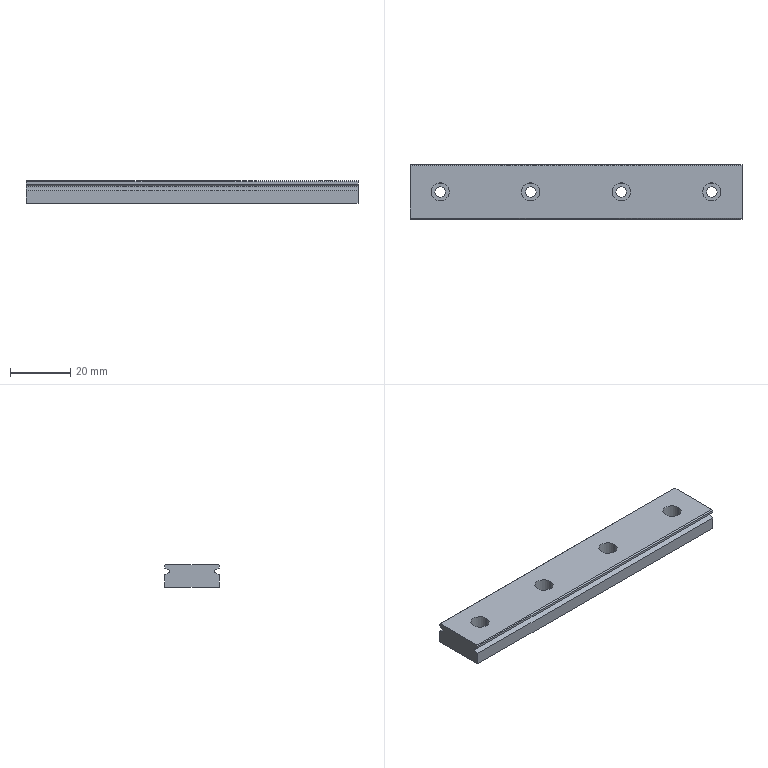Part | SolidWorks | features BaseBody 1, Cut 1 | 1 solid | 36 faces | box 110 x 18 x 7.5 mm | volume 13740 mm3 | plane 20 | cylinder 16 | commonest cylinder face diameters 3.5 x8 6 x8
STEP:
#1=CARTESIAN_POINT('',(-91.75,0.,0.));
#2=VERTEX_POINT('',#1);
#3=CARTESIAN_POINT('',(-88.25,0.,0.));
#4=VERTEX_POINT('',#3);
#5=CARTESIAN_POINT('',(-90.,0.,0.));
#6=DIRECTION('',(0.,0.,1.));
#7=DIRECTION('',(1.,0.,0.));
#8=AXIS2_PLACEMENT_3D('',#5,#6,#7);
#9=CIRCLE('',#8,1.75);
#10=EDGE_CURVE('',#2,#4,#9,.T.);
#11=ORIENTED_EDGE('',*,*,#10,.F.);
#12=CARTESIAN_POINT('',(-91.75,0.,3.));
#13=VERTEX_POINT('',#12);
#14=CARTESIAN_POINT('',(-91.75,0.,-1.163));
#15=DIRECTION('',(0.,0.,1.));
#16=VECTOR('',#15,1000.);
#17=LINE('',#14,#16);
#18=EDGE_CURVE('',#2,#13,#17,.T.);
#19=ORIENTED_EDGE('',*,*,#18,.T.);
#20=CARTESIAN_POINT('',(-88.25,0.,3.));
#21=VERTEX_POINT('',#20);
#22=CARTESIAN_POINT('',(-90.,0.,3.));
#23=DIRECTION('',(0.,0.,-1.));
#24=DIRECTION('',(1.,0.,0.));
#25=AXIS2_PLACEMENT_3D('',#22,#23,#24);
#26=CIRCLE('',#25,1.75);
#27=EDGE_CURVE('',#21,#13,#26,.T.);
#28=ORIENTED_EDGE('',*,*,#27,.F.);
#29=CARTESIAN_POINT('',(-88.25,0.,-1.163));
#30=DIRECTION('',(0.,0.,1.));
#31=VECTOR('',#30,1000.);
#32=LINE('',#29,#31);
#33=EDGE_CURVE('',#4,#21,#32,.T.);
#34=ORIENTED_EDGE('',*,*,#33,.F.);
#35=EDGE_LOOP('',(#11,#19,#28,#34));
#36=FACE_OUTER_BOUND('',#35,.T.);
#37=CARTESIAN_POINT('',(-90.,0.,-1.163));
#38=DIRECTION('',(0.,0.,1.));
#39=DIRECTION('',(1.,0.,0.));
#40=AXIS2_PLACEMENT_3D('',#37,#38,#39);
#41=CYLINDRICAL_SURFACE('',#40,1.75);
#42=ADVANCED_FACE('',(#36),#41,.F.);
#43=CARTESIAN_POINT('',(-61.75,0.,0.));
#44=VERTEX_POINT('',#43);
#45=CARTESIAN_POINT('',(-58.25,0.,0.));
#46=VERTEX_POINT('',#45);
#47=CARTESIAN_POINT('',(-60.,0.,0.));
#48=DIRECTION('',(0.,0.,1.));
#49=DIRECTION('',(1.,0.,0.));
#50=AXIS2_PLACEMENT_3D('',#47,#48,#49);
#51=CIRCLE('',#50,1.75);
#52=EDGE_CURVE('',#44,#46,#51,.T.);
#53=ORIENTED_EDGE('',*,*,#52,.F.);
#54=CARTESIAN_POINT('',(-61.75,0.,3.));
#55=VERTEX_POINT('',#54);
#56=CARTESIAN_POINT('',(-61.75,0.,-1.163));
#57=DIRECTION('',(0.,0.,1.));
#58=VECTOR('',#57,1000.);
#59=LINE('',#56,#58);
#60=EDGE_CURVE('',#44,#55,#59,.T.);
#61=ORIENTED_EDGE('',*,*,#60,.T.);
#62=CARTESIAN_POINT('',(-58.25,0.,3.));
#63=VERTEX_POINT('',#62);
#64=CARTESIAN_POINT('',(-60.,0.,3.));
#65=DIRECTION('',(0.,0.,-1.));
#66=DIRECTION('',(1.,0.,0.));
#67=AXIS2_PLACEMENT_3D('',#64,#65,#66);
#68=CIRCLE('',#67,1.75);
#69=EDGE_CURVE('',#63,#55,#68,.T.);
#70=ORIENTED_EDGE('',*,*,#69,.F.);
#71=CARTESIAN_POINT('',(-58.25,0.,-1.163));
#72=DIRECTION('',(0.,0.,1.));
#73=VECTOR('',#72,1000.);
#74=LINE('',#71,#73);
#75=EDGE_CURVE('',#46,#63,#74,.T.);
#76=ORIENTED_EDGE('',*,*,#75,.F.);
#77=EDGE_LOOP('',(#53,#61,#70,#76));
#78=FACE_OUTER_BOUND('',#77,.T.);
#79=CARTESIAN_POINT('',(-60.,0.,-1.163));
#80=DIRECTION('',(0.,0.,1.));
#81=DIRECTION('',(1.,0.,0.));
#82=AXIS2_PLACEMENT_3D('',#79,#80,#81);
#83=CYLINDRICAL_SURFACE('',#82,1.75);
#84=ADVANCED_FACE('',(#78),#83,.F.);
#85=CARTESIAN_POINT('',(-31.75,0.,0.));
#86=VERTEX_POINT('',#85);
#87=CARTESIAN_POINT('',(-28.25,0.,0.));
#88=VERTEX_POINT('',#87);
#89=CARTESIAN_POINT('',(-30.,0.,0.));
#90=DIRECTION('',(0.,0.,1.));
#91=DIRECTION('',(1.,0.,0.));
#92=AXIS2_PLACEMENT_3D('',#89,#90,#91);
#93=CIRCLE('',#92,1.75);
#94=EDGE_CURVE('',#86,#88,#93,.T.);
#95=ORIENTED_EDGE('',*,*,#94,.F.);
#96=CARTESIAN_POINT('',(-31.75,0.,3.));
#97=VERTEX_POINT('',#96);
#98=CARTESIAN_POINT('',(-31.75,0.,-1.163));
#99=DIRECTION('',(0.,0.,1.));
#100=VECTOR('',#99,1000.);
#101=LINE('',#98,#100);
#102=EDGE_CURVE('',#86,#97,#101,.T.);
#103=ORIENTED_EDGE('',*,*,#102,.T.);
#104=CARTESIAN_POINT('',(-28.25,0.,3.));
#105=VERTEX_POINT('',#104);
#106=CARTESIAN_POINT('',(-30.,0.,3.));
#107=DIRECTION('',(0.,0.,-1.));
#108=DIRECTION('',(1.,0.,0.));
#109=AXIS2_PLACEMENT_3D('',#106,#107,#108);
#110=CIRCLE('',#109,1.75);
#111=EDGE_CURVE('',#105,#97,#110,.T.);
#112=ORIENTED_EDGE('',*,*,#111,.F.);
#113=CARTESIAN_POINT('',(-28.25,0.,-1.163));
#114=DIRECTION('',(0.,0.,1.));
#115=VECTOR('',#114,1000.);
#116=LINE('',#113,#115);
#117=EDGE_CURVE('',#88,#105,#116,.T.);
#118=ORIENTED_EDGE('',*,*,#117,.F.);
#119=EDGE_LOOP('',(#95,#103,#112,#118));
#120=FACE_OUTER_BOUND('',#119,.T.);
#121=CARTESIAN_POINT('',(-30.,0.,-1.163));
#122=DIRECTION('',(0.,0.,1.));
#123=DIRECTION('',(1.,0.,0.));
#124=AXIS2_PLACEMENT_3D('',#121,#122,#123);
#125=CYLINDRICAL_SURFACE('',#124,1.75);
#126=ADVANCED_FACE('',(#120),#125,.F.);
#127=CARTESIAN_POINT('',(-1.75,0.,0.));
#128=VERTEX_POINT('',#127);
#129=CARTESIAN_POINT('',(1.75,0.,0.));
#130=VERTEX_POINT('',#129);
#131=CARTESIAN_POINT('',(0.,0.,0.));
#132=DIRECTION('',(0.,0.,1.));
#133=DIRECTION('',(1.,0.,0.));
#134=AXIS2_PLACEMENT_3D('',#131,#132,#133);
#135=CIRCLE('',#134,1.75);
#136=EDGE_CURVE('',#128,#130,#135,.T.);
#137=ORIENTED_EDGE('',*,*,#136,.F.);
#138=CARTESIAN_POINT('',(-1.75,0.,3.));
#139=VERTEX_POINT('',#138);
#140=CARTESIAN_POINT('',(-1.75,0.,1.5));
#141=DIRECTION('',(0.,0.,1.));
#142=VECTOR('',#141,1000.);
#143=LINE('',#140,#142);
#144=EDGE_CURVE('',#128,#139,#143,.T.);
#145=ORIENTED_EDGE('',*,*,#144,.T.);
#146=CARTESIAN_POINT('',(1.75,0.,3.));
#147=VERTEX_POINT('',#146);
#148=CARTESIAN_POINT('',(0.,0.,3.));
#149=DIRECTION('',(0.,0.,-1.));
#150=DIRECTION('',(1.,0.,0.));
#151=AXIS2_PLACEMENT_3D('',#148,#149,#150);
#152=CIRCLE('',#151,1.75);
#153=EDGE_CURVE('',#147,#139,#152,.T.);
#154=ORIENTED_EDGE('',*,*,#153,.F.);
#155=CARTESIAN_POINT('',(1.75,0.,1.5));
#156=DIRECTION('',(0.,0.,1.));
#157=VECTOR('',#156,1000.);
#158=LINE('',#155,#157);
#159=EDGE_CURVE('',#130,#147,#158,.T.);
#160=ORIENTED_EDGE('',*,*,#159,.F.);
#161=EDGE_LOOP('',(#137,#145,#154,#160));
#162=FACE_OUTER_BOUND('',#161,.T.);
#163=CARTESIAN_POINT('',(0.,0.,1.5));
#164=DIRECTION('',(0.,0.,1.));
#165=DIRECTION('',(1.,0.,0.));
#166=AXIS2_PLACEMENT_3D('',#163,#164,#165);
#167=CYLINDRICAL_SURFACE('',#166,1.75);
#168=ADVANCED_FACE('',(#162),#167,.F.);
#169=CARTESIAN_POINT('',(-93.,0.,3.));
#170=VERTEX_POINT('',#169);
#171=CARTESIAN_POINT('',(-87.,0.,3.));
#172=VERTEX_POINT('',#171);
#173=CARTESIAN_POINT('',(-90.,0.,3.));
#174=DIRECTION('',(0.,0.,1.));
#175=DIRECTION('',(1.,0.,0.));
#176=AXIS2_PLACEMENT_3D('',#173,#174,#175);
#177=CIRCLE('',#176,3.);
#178=EDGE_CURVE('',#170,#172,#177,.T.);
#179=ORIENTED_EDGE('',*,*,#178,.F.);
#180=CARTESIAN_POINT('',(-93.,0.,7.5));
#181=VERTEX_POINT('',#180);
#182=CARTESIAN_POINT('',(-93.,0.,-1.163));
#183=DIRECTION('',(0.,0.,1.));
#184=VECTOR('',#183,1000.);
#185=LINE('',#182,#184);
#186=EDGE_CURVE('',#170,#181,#185,.T.);
#187=ORIENTED_EDGE('',*,*,#186,.T.);
#188=CARTESIAN_POINT('',(-87.,0.,7.5));
#189=VERTEX_POINT('',#188);
#190=CARTESIAN_POINT('',(-90.,0.,7.5));
#191=DIRECTION('',(0.,0.,-1.));
#192=DIRECTION('',(1.,0.,0.));
#193=AXIS2_PLACEMENT_3D('',#190,#191,#192);
#194=CIRCLE('',#193,3.);
#195=EDGE_CURVE('',#189,#181,#194,.T.);
#196=ORIENTED_EDGE('',*,*,#195,.F.);
#197=CARTESIAN_POINT('',(-87.,0.,-1.163));
#198=DIRECTION('',(0.,0.,1.));
#199=VECTOR('',#198,1000.);
#200=LINE('',#197,#199);
#201=EDGE_CURVE('',#172,#189,#200,.T.);
#202=ORIENTED_EDGE('',*,*,#201,.F.);
#203=EDGE_LOOP('',(#179,#187,#196,#202));
#204=FACE_OUTER_BOUND('',#203,.T.);
#205=CARTESIAN_POINT('',(-90.,0.,-1.163));
#206=DIRECTION('',(0.,0.,1.));
#207=DIRECTION('',(1.,0.,0.));
#208=AXIS2_PLACEMENT_3D('',#205,#206,#207);
#209=CYLINDRICAL_SURFACE('',#208,3.);
#210=ADVANCED_FACE('',(#204),#209,.F.);
#211=CARTESIAN_POINT('',(-63.,0.,3.));
#212=VERTEX_POINT('',#211);
#213=CARTESIAN_POINT('',(-57.,0.,3.));
#214=VERTEX_POINT('',#213);
#215=CARTESIAN_POINT('',(-60.,0.,3.));
#216=DIRECTION('',(0.,0.,1.));
#217=DIRECTION('',(1.,0.,0.));
#218=AXIS2_PLACEMENT_3D('',#215,#216,#217);
#219=CIRCLE('',#218,3.);
#220=EDGE_CURVE('',#212,#214,#219,.T.);
#221=ORIENTED_EDGE('',*,*,#220,.F.);
#222=CARTESIAN_POINT('',(-63.,0.,7.5));
#223=VERTEX_POINT('',#222);
#224=CARTESIAN_POINT('',(-63.,0.,-1.163));
#225=DIRECTION('',(0.,0.,1.));
#226=VECTOR('',#225,1000.);
#227=LINE('',#224,#226);
#228=EDGE_CURVE('',#212,#223,#227,.T.);
#229=ORIENTED_EDGE('',*,*,#228,.T.);
#230=CARTESIAN_POINT('',(-57.,0.,7.5));
#231=VERTEX_POINT('',#230);
#232=CARTESIAN_POINT('',(-60.,0.,7.5));
#233=DIRECTION('',(0.,0.,-1.));
#234=DIRECTION('',(1.,0.,0.));
#235=AXIS2_PLACEMENT_3D('',#232,#233,#234);
#236=CIRCLE('',#235,3.);
#237=EDGE_CURVE('',#231,#223,#236,.T.);
#238=ORIENTED_EDGE('',*,*,#237,.F.);
#239=CARTESIAN_POINT('',(-57.,0.,-1.163));
#240=DIRECTION('',(0.,0.,1.));
#241=VECTOR('',#240,1000.);
#242=LINE('',#239,#241);
#243=EDGE_CURVE('',#214,#231,#242,.T.);
#244=ORIENTED_EDGE('',*,*,#243,.F.);
#245=EDGE_LOOP('',(#221,#229,#238,#244));
#246=FACE_OUTER_BOUND('',#245,.T.);
#247=CARTESIAN_POINT('',(-60.,0.,-1.163));
#248=DIRECTION('',(0.,0.,1.));
#249=DIRECTION('',(1.,0.,0.));
#250=AXIS2_PLACEMENT_3D('',#247,#248,#249);
#251=CYLINDRICAL_SURFACE('',#250,3.);
#252=ADVANCED_FACE('',(#246),#251,.F.);
#253=CARTESIAN_POINT('',(-33.,0.,3.));
#254=VERTEX_POINT('',#253);
#255=CARTESIAN_POINT('',(-27.,0.,3.));
#256=VERTEX_POINT('',#255);
#257=CARTESIAN_POINT('',(-30.,0.,3.));
#258=DIRECTION('',(0.,0.,1.));
#259=DIRECTION('',(1.,0.,0.));
#260=AXIS2_PLACEMENT_3D('',#257,#258,#259);
#261=CIRCLE('',#260,3.);
#262=EDGE_CURVE('',#254,#256,#261,.T.);
#263=ORIENTED_EDGE('',*,*,#262,.F.);
#264=CARTESIAN_POINT('',(-33.,0.,7.5));
#265=VERTEX_POINT('',#264);
#266=CARTESIAN_POINT('',(-33.,0.,-1.163));
#267=DIRECTION('',(0.,0.,1.));
#268=VECTOR('',#267,1000.);
#269=LINE('',#266,#268);
#270=EDGE_CURVE('',#254,#265,#269,.T.);
#271=ORIENTED_EDGE('',*,*,#270,.T.);
#272=CARTESIAN_POINT('',(-27.,0.,7.5));
#273=VERTEX_POINT('',#272);
#274=CARTESIAN_POINT('',(-30.,0.,7.5));
#275=DIRECTION('',(0.,0.,-1.));
#276=DIRECTION('',(1.,0.,0.));
#277=AXIS2_PLACEMENT_3D('',#274,#275,#276);
#278=CIRCLE('',#277,3.);
#279=EDGE_CURVE('',#273,#265,#278,.T.);
#280=ORIENTED_EDGE('',*,*,#279,.F.);
#281=CARTESIAN_POINT('',(-27.,0.,-1.163));
#282=DIRECTION('',(0.,0.,1.));
#283=VECTOR('',#282,1000.);
#284=LINE('',#281,#283);
#285=EDGE_CURVE('',#256,#273,#284,.T.);
#286=ORIENTED_EDGE('',*,*,#285,.F.);
#287=EDGE_LOOP('',(#263,#271,#280,#286));
#288=FACE_OUTER_BOUND('',#287,.T.);
#289=CARTESIAN_POINT('',(-30.,0.,-1.163));
#290=DIRECTION('',(0.,0.,1.));
#291=DIRECTION('',(1.,0.,0.));
#292=AXIS2_PLACEMENT_3D('',#289,#290,#291);
#293=CYLINDRICAL_SURFACE('',#292,3.);
#294=ADVANCED_FACE('',(#288),#293,.F.);
#295=CARTESIAN_POINT('',(3.,0.,7.5));
#296=VERTEX_POINT('',#295);
#297=CARTESIAN_POINT('',(-3.,0.,7.5));
#298=VERTEX_POINT('',#297);
#299=CARTESIAN_POINT('',(0.,0.,7.5));
#300=DIRECTION('',(0.,0.,-1.));
#301=DIRECTION('',(-1.,0.,0.));
#302=AXIS2_PLACEMENT_3D('',#299,#300,#301);
#303=CIRCLE('',#302,3.);
#304=EDGE_CURVE('',#296,#298,#303,.T.);
#305=ORIENTED_EDGE('',*,*,#304,.F.);
#306=CARTESIAN_POINT('',(3.,0.,3.));
#307=VERTEX_POINT('',#306);
#308=CARTESIAN_POINT('',(3.,0.,5.25));
#309=DIRECTION('',(0.,0.,-1.));
#310=VECTOR('',#309,1000.);
#311=LINE('',#308,#310);
#312=EDGE_CURVE('',#296,#307,#311,.T.);
#313=ORIENTED_EDGE('',*,*,#312,.T.);
#314=CARTESIAN_POINT('',(-3.,0.,3.));
#315=VERTEX_POINT('',#314);
#316=CARTESIAN_POINT('',(0.,0.,3.));
#317=DIRECTION('',(0.,0.,-1.));
#318=DIRECTION('',(-1.,0.,0.));
#319=AXIS2_PLACEMENT_3D('',#316,#317,#318);
#320=CIRCLE('',#319,3.);
#321=EDGE_CURVE('',#307,#315,#320,.T.);
#322=ORIENTED_EDGE('',*,*,#321,.T.);
#323=CARTESIAN_POINT('',(-3.,0.,5.25));
#324=DIRECTION('',(0.,0.,-1.));
#325=VECTOR('',#324,1000.);
#326=LINE('',#323,#325);
#327=EDGE_CURVE('',#298,#315,#326,.T.);
#328=ORIENTED_EDGE('',*,*,#327,.F.);
#329=EDGE_LOOP('',(#305,#313,#322,#328));
#330=FACE_OUTER_BOUND('',#329,.T.);
#331=CARTESIAN_POINT('',(0.,0.,5.25));
#332=DIRECTION('',(0.,0.,-1.));
#333=DIRECTION('',(-1.,0.,0.));
#334=AXIS2_PLACEMENT_3D('',#331,#332,#333);
#335=CYLINDRICAL_SURFACE('',#334,3.);
#336=ADVANCED_FACE('',(#330),#335,.F.);
#337=CARTESIAN_POINT('',(10.,-9.,0.));
#338=VERTEX_POINT('',#337);
#339=CARTESIAN_POINT('',(10.,9.,0.));
#340=VERTEX_POINT('',#339);
#341=CARTESIAN_POINT('',(10.,0.,0.));
#342=DIRECTION('',(0.,1.,0.));
#343=VECTOR('',#342,1000.);
#344=LINE('',#341,#343);
#345=EDGE_CURVE('',#338,#340,#344,.T.);
#346=ORIENTED_EDGE('',*,*,#345,.F.);
#347=CARTESIAN_POINT('',(-100.,-9.,0.));
#348=VERTEX_POINT('',#347);
#349=CARTESIAN_POINT('',(-10.,-9.,0.));
#350=DIRECTION('',(-1.,0.,0.));
#351=VECTOR('',#350,1000.);
#352=LINE('',#349,#351);
#353=EDGE_CURVE('',#338,#348,#352,.T.);
#354=ORIENTED_EDGE('',*,*,#353,.T.);
#355=CARTESIAN_POINT('',(-100.,9.,0.));
#356=VERTEX_POINT('',#355);
#357=CARTESIAN_POINT('',(-100.,0.,0.));
#358=DIRECTION('',(0.,1.,0.));
#359=VECTOR('',#358,1000.);
#360=LINE('',#357,#359);
#361=EDGE_CURVE('',#348,#356,#360,.T.);
#362=ORIENTED_EDGE('',*,*,#361,.T.);
#363=CARTESIAN_POINT('',(-10.,9.,0.));
#364=DIRECTION('',(1.,0.,0.));
#365=VECTOR('',#364,1000.);
#366=LINE('',#363,#365);
#367=EDGE_CURVE('',#356,#340,#366,.T.);
#368=ORIENTED_EDGE('',*,*,#367,.T.);
#369=EDGE_LOOP('',(#346,#354,#362,#368));
#370=FACE_OUTER_BOUND('',#369,.T.);
#371=CARTESIAN_POINT('',(-90.,0.,0.));
#372=DIRECTION('',(0.,0.,1.));
#373=DIRECTION('',(1.,0.,0.));
#374=AXIS2_PLACEMENT_3D('',#371,#372,#373);
#375=CIRCLE('',#374,1.75);
#376=EDGE_CURVE('',#4,#2,#375,.T.);
#377=ORIENTED_EDGE('',*,*,#376,.T.);
#378=ORIENTED_EDGE('',*,*,#10,.T.);
#379=EDGE_LOOP('',(#377,#378));
#380=FACE_BOUND('',#379,.T.);
#381=CARTESIAN_POINT('',(-60.,0.,0.));
#382=DIRECTION('',(0.,0.,1.));
#383=DIRECTION('',(1.,0.,0.));
#384=AXIS2_PLACEMENT_3D('',#381,#382,#383);
#385=CIRCLE('',#384,1.75);
#386=EDGE_CURVE('',#46,#44,#385,.T.);
#387=ORIENTED_EDGE('',*,*,#386,.T.);
#388=ORIENTED_EDGE('',*,*,#52,.T.);
#389=EDGE_LOOP('',(#387,#388));
#390=FACE_BOUND('',#389,.T.);
#391=CARTESIAN_POINT('',(-30.,0.,0.));
#392=DIRECTION('',(0.,0.,1.));
#393=DIRECTION('',(1.,0.,0.));
#394=AXIS2_PLACEMENT_3D('',#391,#392,#393);
#395=CIRCLE('',#394,1.75);
#396=EDGE_CURVE('',#88,#86,#395,.T.);
#397=ORIENTED_EDGE('',*,*,#396,.T.);
#398=ORIENTED_EDGE('',*,*,#94,.T.);
#399=EDGE_LOOP('',(#397,#398));
#400=FACE_BOUND('',#399,.T.);
#401=CARTESIAN_POINT('',(0.,0.,0.));
#402=DIRECTION('',(0.,0.,1.));
#403=DIRECTION('',(1.,0.,0.));
#404=AXIS2_PLACEMENT_3D('',#401,#402,#403);
#405=CIRCLE('',#404,1.75);
#406=EDGE_CURVE('',#130,#128,#405,.T.);
#407=ORIENTED_EDGE('',*,*,#406,.T.);
#408=ORIENTED_EDGE('',*,*,#136,.T.);
#409=EDGE_LOOP('',(#407,#408));
#410=FACE_BOUND('',#409,.T.);
#411=CARTESIAN_POINT('',(-10.,0.,0.));
#412=DIRECTION('',(0.,0.,-1.));
#413=DIRECTION('',(-1.,0.,0.));
#414=AXIS2_PLACEMENT_3D('',#411,#412,#413);
#415=PLANE('',#414);
#416=ADVANCED_FACE('',(#370,#380,#390,#400,#410),#415,.T.);
#417=ORIENTED_EDGE('',*,*,#18,.F.);
#418=ORIENTED_EDGE('',*,*,#376,.F.);
#419=ORIENTED_EDGE('',*,*,#33,.T.);
#420=CARTESIAN_POINT('',(-90.,0.,3.));
#421=DIRECTION('',(0.,0.,-1.));
#422=DIRECTION('',(1.,0.,0.));
#423=AXIS2_PLACEMENT_3D('',#420,#421,#422);
#424=CIRCLE('',#423,1.75);
#425=EDGE_CURVE('',#13,#21,#424,.T.);
#426=ORIENTED_EDGE('',*,*,#425,.F.);
#427=EDGE_LOOP('',(#417,#418,#419,#426));
#428=FACE_OUTER_BOUND('',#427,.T.);
#429=CARTESIAN_POINT('',(-90.,0.,-1.163));
#430=DIRECTION('',(0.,0.,1.));
#431=DIRECTION('',(1.,0.,0.));
#432=AXIS2_PLACEMENT_3D('',#429,#430,#431);
#433=CYLINDRICAL_SURFACE('',#432,1.75);
#434=ADVANCED_FACE('',(#428),#433,.F.);
#435=ORIENTED_EDGE('',*,*,#60,.F.);
#436=ORIENTED_EDGE('',*,*,#386,.F.);
#437=ORIENTED_EDGE('',*,*,#75,.T.);
#438=CARTESIAN_POINT('',(-60.,0.,3.));
#439=DIRECTION('',(0.,0.,-1.));
#440=DIRECTION('',(1.,0.,0.));
#441=AXIS2_PLACEMENT_3D('',#438,#439,#440);
#442=CIRCLE('',#441,1.75);
#443=EDGE_CURVE('',#55,#63,#442,.T.);
#444=ORIENTED_EDGE('',*,*,#443,.F.);
#445=EDGE_LOOP('',(#435,#436,#437,#444));
#446=FACE_OUTER_BOUND('',#445,.T.);
#447=CARTESIAN_POINT('',(-60.,0.,-1.163));
#448=DIRECTION('',(0.,0.,1.));
#449=DIRECTION('',(1.,0.,0.));
#450=AXIS2_PLACEMENT_3D('',#447,#448,#449);
#451=CYLINDRICAL_SURFACE('',#450,1.75);
#452=ADVANCED_FACE('',(#446),#451,.F.);
#453=ORIENTED_EDGE('',*,*,#102,.F.);
#454=ORIENTED_EDGE('',*,*,#396,.F.);
#455=ORIENTED_EDGE('',*,*,#117,.T.);
#456=CARTESIAN_POINT('',(-30.,0.,3.));
#457=DIRECTION('',(0.,0.,-1.));
#458=DIRECTION('',(1.,0.,0.));
#459=AXIS2_PLACEMENT_3D('',#456,#457,#458);
#460=CIRCLE('',#459,1.75);
#461=EDGE_CURVE('',#97,#105,#460,.T.);
#462=ORIENTED_EDGE('',*,*,#461,.F.);
#463=EDGE_LOOP('',(#453,#454,#455,#462));
#464=FACE_OUTER_BOUND('',#463,.T.);
#465=CARTESIAN_POINT('',(-30.,0.,-1.163));
#466=DIRECTION('',(0.,0.,1.));
#467=DIRECTION('',(1.,0.,0.));
#468=AXIS2_PLACEMENT_3D('',#465,#466,#467);
#469=CYLINDRICAL_SURFACE('',#468,1.75);
#470=ADVANCED_FACE('',(#464),#469,.F.);
#471=ORIENTED_EDGE('',*,*,#144,.F.);
#472=ORIENTED_EDGE('',*,*,#406,.F.);
#473=ORIENTED_EDGE('',*,*,#159,.T.);
#474=CARTESIAN_POINT('',(0.,0.,3.));
#475=DIRECTION('',(0.,0.,-1.));
#476=DIRECTION('',(1.,0.,0.));
#477=AXIS2_PLACEMENT_3D('',#474,#475,#476);
#478=CIRCLE('',#477,1.75);
#479=EDGE_CURVE('',#139,#147,#478,.T.);
#480=ORIENTED_EDGE('',*,*,#479,.F.);
#481=EDGE_LOOP('',(#471,#472,#473,#480));
#482=FACE_OUTER_BOUND('',#481,.T.);
#483=CARTESIAN_POINT('',(0.,0.,1.5));
#484=DIRECTION('',(0.,0.,1.));
#485=DIRECTION('',(1.,0.,0.));
#486=AXIS2_PLACEMENT_3D('',#483,#484,#485);
#487=CYLINDRICAL_SURFACE('',#486,1.75);
#488=ADVANCED_FACE('',(#482),#487,.F.);
#489=CARTESIAN_POINT('',(10.,9.,4.2));
#490=VERTEX_POINT('',#489);
#491=CARTESIAN_POINT('',(10.,9.,4.2));
#492=DIRECTION('',(0.,0.,1.));
#493=VECTOR('',#492,1000.);
#494=LINE('',#491,#493);
#495=EDGE_CURVE('',#340,#490,#494,.T.);
#496=ORIENTED_EDGE('',*,*,#495,.F.);
#497=ORIENTED_EDGE('',*,*,#367,.F.);
#498=CARTESIAN_POINT('',(-100.,9.,4.2));
#499=VERTEX_POINT('',#498);
#500=CARTESIAN_POINT('',(-100.,9.,4.2));
#501=DIRECTION('',(0.,0.,1.));
#502=VECTOR('',#501,1000.);
#503=LINE('',#500,#502);
#504=EDGE_CURVE('',#356,#499,#503,.T.);
#505=ORIENTED_EDGE('',*,*,#504,.T.);
#506=CARTESIAN_POINT('',(-10.,9.,4.2));
#507=DIRECTION('',(1.,0.,0.));
#508=VECTOR('',#507,1000.);
#509=LINE('',#506,#508);
#510=EDGE_CURVE('',#499,#490,#509,.T.);
#511=ORIENTED_EDGE('',*,*,#510,.T.);
#512=EDGE_LOOP('',(#496,#497,#505,#511));
#513=FACE_OUTER_BOUND('',#512,.T.);
#514=CARTESIAN_POINT('',(-10.,9.,4.2));
#515=DIRECTION('',(0.,1.,0.));
#516=DIRECTION('',(0.,0.,1.));
#517=AXIS2_PLACEMENT_3D('',#514,#515,#516);
#518=PLANE('',#517);
#519=ADVANCED_FACE('',(#513),#518,.T.);
#520=ORIENTED_EDGE('',*,*,#504,.F.);
#521=ORIENTED_EDGE('',*,*,#361,.F.);
#522=CARTESIAN_POINT('',(-100.,-9.,4.2));
#523=VERTEX_POINT('',#522);
#524=CARTESIAN_POINT('',(-100.,-9.,0.));
#525=DIRECTION('',(0.,0.,1.));
#526=VECTOR('',#525,1000.);
#527=LINE('',#524,#526);
#528=EDGE_CURVE('',#348,#523,#527,.T.);
#529=ORIENTED_EDGE('',*,*,#528,.T.);
#530=CARTESIAN_POINT('',(-100.,-7.5,4.95));
#531=VERTEX_POINT('',#530);
#532=CARTESIAN_POINT('',(-100.,-9.,4.2));
#533=DIRECTION('',(0.,-0.8944,-0.4472));
#534=VECTOR('',#533,1000.);
#535=LINE('',#532,#534);
#536=EDGE_CURVE('',#531,#523,#535,.T.);
#537=ORIENTED_EDGE('',*,*,#536,.F.);
#538=CARTESIAN_POINT('',(-100.,-7.5,5.625));
#539=VERTEX_POINT('',#538);
#540=CARTESIAN_POINT('',(-100.,-7.5,4.95));
#541=DIRECTION('',(0.,0.,-1.));
#542=VECTOR('',#541,1000.);
#543=LINE('',#540,#542);
#544=EDGE_CURVE('',#539,#531,#543,.T.);
#545=ORIENTED_EDGE('',*,*,#544,.F.);
#546=CARTESIAN_POINT('',(-100.,-9.,6.375));
#547=VERTEX_POINT('',#546);
#548=CARTESIAN_POINT('',(-100.,-7.5,5.625));
#549=DIRECTION('',(0.,0.8944,-0.4472));
#550=VECTOR('',#549,1000.);
#551=LINE('',#548,#550);
#552=EDGE_CURVE('',#547,#539,#551,.T.);
#553=ORIENTED_EDGE('',*,*,#552,.F.);
#554=CARTESIAN_POINT('',(-100.,-9.,7.125));
#555=VERTEX_POINT('',#554);
#556=CARTESIAN_POINT('',(-100.,-9.,6.375));
#557=DIRECTION('',(0.,0.,-1.));
#558=VECTOR('',#557,1000.);
#559=LINE('',#556,#558);
#560=EDGE_CURVE('',#555,#547,#559,.T.);
#561=ORIENTED_EDGE('',*,*,#560,.F.);
#562=CARTESIAN_POINT('',(-100.,-8.625,7.5));
#563=VERTEX_POINT('',#562);
#564=CARTESIAN_POINT('',(-100.,-9.,7.125));
#565=DIRECTION('',(0.,-0.7071,-0.7071));
#566=VECTOR('',#565,1000.);
#567=LINE('',#564,#566);
#568=EDGE_CURVE('',#563,#555,#567,.T.);
#569=ORIENTED_EDGE('',*,*,#568,.F.);
#570=CARTESIAN_POINT('',(-100.,8.625,7.5));
#571=VERTEX_POINT('',#570);
#572=CARTESIAN_POINT('',(-100.,0.,7.5));
#573=DIRECTION('',(0.,1.,0.));
#574=VECTOR('',#573,1000.);
#575=LINE('',#572,#574);
#576=EDGE_CURVE('',#563,#571,#575,.T.);
#577=ORIENTED_EDGE('',*,*,#576,.T.);
#578=CARTESIAN_POINT('',(-100.,9.,7.125));
#579=VERTEX_POINT('',#578);
#580=CARTESIAN_POINT('',(-100.,8.625,7.5));
#581=DIRECTION('',(0.,-0.7071,0.7071));
#582=VECTOR('',#581,1000.);
#583=LINE('',#580,#582);
#584=EDGE_CURVE('',#579,#571,#583,.T.);
#585=ORIENTED_EDGE('',*,*,#584,.F.);
#586=CARTESIAN_POINT('',(-100.,9.,6.375));
#587=VERTEX_POINT('',#586);
#588=CARTESIAN_POINT('',(-100.,9.,7.125));
#589=DIRECTION('',(0.,0.,1.));
#590=VECTOR('',#589,1000.);
#591=LINE('',#588,#590);
#592=EDGE_CURVE('',#587,#579,#591,.T.);
#593=ORIENTED_EDGE('',*,*,#592,.F.);
#594=CARTESIAN_POINT('',(-100.,7.5,5.625));
#595=VERTEX_POINT('',#594);
#596=CARTESIAN_POINT('',(-100.,9.,6.375));
#597=DIRECTION('',(0.,0.8944,0.4472));
#598=VECTOR('',#597,1000.);
#599=LINE('',#596,#598);
#600=EDGE_CURVE('',#595,#587,#599,.T.);
#601=ORIENTED_EDGE('',*,*,#600,.F.);
#602=CARTESIAN_POINT('',(-100.,7.5,4.95));
#603=VERTEX_POINT('',#602);
#604=CARTESIAN_POINT('',(-100.,7.5,5.625));
#605=DIRECTION('',(0.,0.,1.));
#606=VECTOR('',#605,1000.);
#607=LINE('',#604,#606);
#608=EDGE_CURVE('',#603,#595,#607,.T.);
#609=ORIENTED_EDGE('',*,*,#608,.F.);
#610=CARTESIAN_POINT('',(-100.,7.5,4.95));
#611=DIRECTION('',(0.,0.8944,-0.4472));
#612=VECTOR('',#611,1000.);
#613=LINE('',#610,#612);
#614=EDGE_CURVE('',#603,#499,#613,.T.);
#615=ORIENTED_EDGE('',*,*,#614,.T.);
#616=EDGE_LOOP('',(#520,#521,#529,#537,#545,#553,#561,#569,#577,#585,#593,#601,#609,#615));
#617=FACE_OUTER_BOUND('',#616,.T.);
#618=CARTESIAN_POINT('',(-100.,0.,0.));
#619=DIRECTION('',(-1.,0.,0.));
#620=DIRECTION('',(0.,0.,1.));
#621=AXIS2_PLACEMENT_3D('',#618,#619,#620);
#622=PLANE('',#621);
#623=ADVANCED_FACE('',(#617),#622,.T.);
#624=CARTESIAN_POINT('',(10.,-9.,4.2));
#625=VERTEX_POINT('',#624);
#626=CARTESIAN_POINT('',(10.,-9.,0.));
#627=DIRECTION('',(0.,0.,-1.));
#628=VECTOR('',#627,1000.);
#629=LINE('',#626,#628);
#630=EDGE_CURVE('',#625,#338,#629,.T.);
#631=ORIENTED_EDGE('',*,*,#630,.F.);
#632=CARTESIAN_POINT('',(-10.,-9.,4.2));
#633=DIRECTION('',(-1.,0.,0.));
#634=VECTOR('',#633,1000.);
#635=LINE('',#632,#634);
#636=EDGE_CURVE('',#625,#523,#635,.T.);
#637=ORIENTED_EDGE('',*,*,#636,.T.);
#638=ORIENTED_EDGE('',*,*,#528,.F.);
#639=ORIENTED_EDGE('',*,*,#353,.F.);
#640=EDGE_LOOP('',(#631,#637,#638,#639));
#641=FACE_OUTER_BOUND('',#640,.T.);
#642=CARTESIAN_POINT('',(-10.,-9.,0.));
#643=DIRECTION('',(0.,-1.,0.));
#644=DIRECTION('',(0.,0.,-1.));
#645=AXIS2_PLACEMENT_3D('',#642,#643,#644);
#646=PLANE('',#645);
#647=ADVANCED_FACE('',(#641),#646,.T.);
#648=ORIENTED_EDGE('',*,*,#27,.T.);
#649=ORIENTED_EDGE('',*,*,#425,.T.);
#650=EDGE_LOOP('',(#648,#649));
#651=FACE_BOUND('',#650,.T.);
#652=CARTESIAN_POINT('',(-90.,0.,3.));
#653=DIRECTION('',(0.,0.,1.));
#654=DIRECTION('',(1.,0.,0.));
#655=AXIS2_PLACEMENT_3D('',#652,#653,#654);
#656=CIRCLE('',#655,3.);
#657=EDGE_CURVE('',#172,#170,#656,.T.);
#658=ORIENTED_EDGE('',*,*,#657,.T.);
#659=ORIENTED_EDGE('',*,*,#178,.T.);
#660=EDGE_LOOP('',(#658,#659));
#661=FACE_OUTER_BOUND('',#660,.T.);
#662=CARTESIAN_POINT('',(-90.,0.,3.));
#663=DIRECTION('',(0.,0.,1.));
#664=DIRECTION('',(1.,0.,0.));
#665=AXIS2_PLACEMENT_3D('',#662,#663,#664);
#666=PLANE('',#665);
#667=ADVANCED_FACE('',(#651,#661),#666,.T.);
#668=ORIENTED_EDGE('',*,*,#69,.T.);
#669=ORIENTED_EDGE('',*,*,#443,.T.);
#670=EDGE_LOOP('',(#668,#669));
#671=FACE_BOUND('',#670,.T.);
#672=CARTESIAN_POINT('',(-60.,0.,3.));
#673=DIRECTION('',(0.,0.,1.));
#674=DIRECTION('',(1.,0.,0.));
#675=AXIS2_PLACEMENT_3D('',#672,#673,#674);
#676=CIRCLE('',#675,3.);
#677=EDGE_CURVE('',#214,#212,#676,.T.);
#678=ORIENTED_EDGE('',*,*,#677,.T.);
#679=ORIENTED_EDGE('',*,*,#220,.T.);
#680=EDGE_LOOP('',(#678,#679));
#681=FACE_OUTER_BOUND('',#680,.T.);
#682=CARTESIAN_POINT('',(-60.,0.,3.));
#683=DIRECTION('',(0.,0.,1.));
#684=DIRECTION('',(1.,0.,0.));
#685=AXIS2_PLACEMENT_3D('',#682,#683,#684);
#686=PLANE('',#685);
#687=ADVANCED_FACE('',(#671,#681),#686,.T.);
#688=ORIENTED_EDGE('',*,*,#111,.T.);
#689=ORIENTED_EDGE('',*,*,#461,.T.);
#690=EDGE_LOOP('',(#688,#689));
#691=FACE_BOUND('',#690,.T.);
#692=CARTESIAN_POINT('',(-30.,0.,3.));
#693=DIRECTION('',(0.,0.,1.));
#694=DIRECTION('',(1.,0.,0.));
#695=AXIS2_PLACEMENT_3D('',#692,#693,#694);
#696=CIRCLE('',#695,3.);
#697=EDGE_CURVE('',#256,#254,#696,.T.);
#698=ORIENTED_EDGE('',*,*,#697,.T.);
#699=ORIENTED_EDGE('',*,*,#262,.T.);
#700=EDGE_LOOP('',(#698,#699));
#701=FACE_OUTER_BOUND('',#700,.T.);
#702=CARTESIAN_POINT('',(-30.,0.,3.));
#703=DIRECTION('',(0.,0.,1.));
#704=DIRECTION('',(1.,0.,0.));
#705=AXIS2_PLACEMENT_3D('',#702,#703,#704);
#706=PLANE('',#705);
#707=ADVANCED_FACE('',(#691,#701),#706,.T.);
#708=ORIENTED_EDGE('',*,*,#153,.T.);
#709=ORIENTED_EDGE('',*,*,#479,.T.);
#710=EDGE_LOOP('',(#708,#709));
#711=FACE_BOUND('',#710,.T.);
#712=CARTESIAN_POINT('',(0.,0.,3.));
#713=DIRECTION('',(0.,0.,-1.));
#714=DIRECTION('',(-1.,0.,0.));
#715=AXIS2_PLACEMENT_3D('',#712,#713,#714);
#716=CIRCLE('',#715,3.);
#717=EDGE_CURVE('',#315,#307,#716,.T.);
#718=ORIENTED_EDGE('',*,*,#717,.F.);
#719=ORIENTED_EDGE('',*,*,#321,.F.);
#720=EDGE_LOOP('',(#718,#719));
#721=FACE_OUTER_BOUND('',#720,.T.);
#722=CARTESIAN_POINT('',(0.,0.,3.));
#723=DIRECTION('',(0.,0.,-1.));
#724=DIRECTION('',(-1.,0.,0.));
#725=AXIS2_PLACEMENT_3D('',#722,#723,#724);
#726=PLANE('',#725);
#727=ADVANCED_FACE('',(#711,#721),#726,.F.);
#728=CARTESIAN_POINT('',(10.,7.5,4.95));
#729=VERTEX_POINT('',#728);
#730=CARTESIAN_POINT('',(10.,7.5,4.95));
#731=DIRECTION('',(0.,-0.8944,0.4472));
#732=VECTOR('',#731,1000.);
#733=LINE('',#730,#732);
#734=EDGE_CURVE('',#490,#729,#733,.T.);
#735=ORIENTED_EDGE('',*,*,#734,.F.);
#736=ORIENTED_EDGE('',*,*,#510,.F.);
#737=ORIENTED_EDGE('',*,*,#614,.F.);
#738=CARTESIAN_POINT('',(-10.,7.5,4.95));
#739=DIRECTION('',(1.,0.,0.));
#740=VECTOR('',#739,1000.);
#741=LINE('',#738,#740);
#742=EDGE_CURVE('',#603,#729,#741,.T.);
#743=ORIENTED_EDGE('',*,*,#742,.T.);
#744=EDGE_LOOP('',(#735,#736,#737,#743));
#745=FACE_OUTER_BOUND('',#744,.T.);
#746=CARTESIAN_POINT('',(-10.,7.5,4.95));
#747=DIRECTION('',(0.,0.4472,0.8944));
#748=DIRECTION('',(0.,-0.8944,0.4472));
#749=AXIS2_PLACEMENT_3D('',#746,#747,#748);
#750=PLANE('',#749);
#751=ADVANCED_FACE('',(#745),#750,.T.);
#752=CARTESIAN_POINT('',(10.,8.625,7.5));
#753=VERTEX_POINT('',#752);
#754=CARTESIAN_POINT('',(10.,-8.625,7.5));
#755=VERTEX_POINT('',#754);
#756=CARTESIAN_POINT('',(10.,19.873,7.5));
#757=DIRECTION('',(0.,-1.,0.));
#758=VECTOR('',#757,1000.);
#759=LINE('',#756,#758);
#760=EDGE_CURVE('',#753,#755,#759,.T.);
#761=ORIENTED_EDGE('',*,*,#760,.F.);
#762=CARTESIAN_POINT('',(-10.,8.625,7.5));
#763=DIRECTION('',(-1.,0.,0.));
#764=VECTOR('',#763,1000.);
#765=LINE('',#762,#764);
#766=EDGE_CURVE('',#753,#571,#765,.T.);
#767=ORIENTED_EDGE('',*,*,#766,.T.);
#768=ORIENTED_EDGE('',*,*,#576,.F.);
#769=CARTESIAN_POINT('',(-10.,-8.625,7.5));
#770=DIRECTION('',(1.,0.,0.));
#771=VECTOR('',#770,1000.);
#772=LINE('',#769,#771);
#773=EDGE_CURVE('',#563,#755,#772,.T.);
#774=ORIENTED_EDGE('',*,*,#773,.T.);
#775=EDGE_LOOP('',(#761,#767,#768,#774));
#776=FACE_OUTER_BOUND('',#775,.T.);
#777=ORIENTED_EDGE('',*,*,#195,.T.);
#778=CARTESIAN_POINT('',(-90.,0.,7.5));
#779=DIRECTION('',(0.,0.,-1.));
#780=DIRECTION('',(1.,0.,0.));
#781=AXIS2_PLACEMENT_3D('',#778,#779,#780);
#782=CIRCLE('',#781,3.);
#783=EDGE_CURVE('',#181,#189,#782,.T.);
#784=ORIENTED_EDGE('',*,*,#783,.T.);
#785=EDGE_LOOP('',(#777,#784));
#786=FACE_BOUND('',#785,.T.);
#787=ORIENTED_EDGE('',*,*,#237,.T.);
#788=CARTESIAN_POINT('',(-60.,0.,7.5));
#789=DIRECTION('',(0.,0.,-1.));
#790=DIRECTION('',(1.,0.,0.));
#791=AXIS2_PLACEMENT_3D('',#788,#789,#790);
#792=CIRCLE('',#791,3.);
#793=EDGE_CURVE('',#223,#231,#792,.T.);
#794=ORIENTED_EDGE('',*,*,#793,.T.);
#795=EDGE_LOOP('',(#787,#794));
#796=FACE_BOUND('',#795,.T.);
#797=ORIENTED_EDGE('',*,*,#279,.T.);
#798=CARTESIAN_POINT('',(-30.,0.,7.5));
#799=DIRECTION('',(0.,0.,-1.));
#800=DIRECTION('',(1.,0.,0.));
#801=AXIS2_PLACEMENT_3D('',#798,#799,#800);
#802=CIRCLE('',#801,3.);
#803=EDGE_CURVE('',#265,#273,#802,.T.);
#804=ORIENTED_EDGE('',*,*,#803,.T.);
#805=EDGE_LOOP('',(#797,#804));
#806=FACE_BOUND('',#805,.T.);
#807=CARTESIAN_POINT('',(0.,0.,7.5));
#808=DIRECTION('',(0.,0.,-1.));
#809=DIRECTION('',(-1.,0.,0.));
#810=AXIS2_PLACEMENT_3D('',#807,#808,#809);
#811=CIRCLE('',#810,3.);
#812=EDGE_CURVE('',#298,#296,#811,.T.);
#813=ORIENTED_EDGE('',*,*,#812,.T.);
#814=ORIENTED_EDGE('',*,*,#304,.T.);
#815=EDGE_LOOP('',(#813,#814));
#816=FACE_BOUND('',#815,.T.);
#817=CARTESIAN_POINT('',(-10.,-8.625,7.5));
#818=DIRECTION('',(0.,0.,1.));
#819=DIRECTION('',(1.,0.,0.));
#820=AXIS2_PLACEMENT_3D('',#817,#818,#819);
#821=PLANE('',#820);
#822=ADVANCED_FACE('',(#776,#786,#796,#806,#816),#821,.T.);
#823=CARTESIAN_POINT('',(10.,-7.5,4.95));
#824=VERTEX_POINT('',#823);
#825=CARTESIAN_POINT('',(10.,-9.,4.2));
#826=DIRECTION('',(0.,-0.8944,-0.4472));
#827=VECTOR('',#826,1000.);
#828=LINE('',#825,#827);
#829=EDGE_CURVE('',#824,#625,#828,.T.);
#830=ORIENTED_EDGE('',*,*,#829,.F.);
#831=CARTESIAN_POINT('',(-10.,-7.5,4.95));
#832=DIRECTION('',(-1.,0.,0.));
#833=VECTOR('',#832,1000.);
#834=LINE('',#831,#833);
#835=EDGE_CURVE('',#824,#531,#834,.T.);
#836=ORIENTED_EDGE('',*,*,#835,.T.);
#837=ORIENTED_EDGE('',*,*,#536,.T.);
#838=ORIENTED_EDGE('',*,*,#636,.F.);
#839=EDGE_LOOP('',(#830,#836,#837,#838));
#840=FACE_OUTER_BOUND('',#839,.T.);
#841=CARTESIAN_POINT('',(-10.,-9.,4.2));
#842=DIRECTION('',(0.,-0.4472,0.8944));
#843=DIRECTION('',(0.,-0.8944,-0.4472));
#844=AXIS2_PLACEMENT_3D('',#841,#842,#843);
#845=PLANE('',#844);
#846=ADVANCED_FACE('',(#840),#845,.T.);
#847=ORIENTED_EDGE('',*,*,#186,.F.);
#848=ORIENTED_EDGE('',*,*,#657,.F.);
#849=ORIENTED_EDGE('',*,*,#201,.T.);
#850=ORIENTED_EDGE('',*,*,#783,.F.);
#851=EDGE_LOOP('',(#847,#848,#849,#850));
#852=FACE_OUTER_BOUND('',#851,.T.);
#853=CARTESIAN_POINT('',(-90.,0.,-1.163));
#854=DIRECTION('',(0.,0.,1.));
#855=DIRECTION('',(1.,0.,0.));
#856=AXIS2_PLACEMENT_3D('',#853,#854,#855);
#857=CYLINDRICAL_SURFACE('',#856,3.);
#858=ADVANCED_FACE('',(#852),#857,.F.);
#859=ORIENTED_EDGE('',*,*,#228,.F.);
#860=ORIENTED_EDGE('',*,*,#677,.F.);
#861=ORIENTED_EDGE('',*,*,#243,.T.);
#862=ORIENTED_EDGE('',*,*,#793,.F.);
#863=EDGE_LOOP('',(#859,#860,#861,#862));
#864=FACE_OUTER_BOUND('',#863,.T.);
#865=CARTESIAN_POINT('',(-60.,0.,-1.163));
#866=DIRECTION('',(0.,0.,1.));
#867=DIRECTION('',(1.,0.,0.));
#868=AXIS2_PLACEMENT_3D('',#865,#866,#867);
#869=CYLINDRICAL_SURFACE('',#868,3.);
#870=ADVANCED_FACE('',(#864),#869,.F.);
#871=ORIENTED_EDGE('',*,*,#270,.F.);
#872=ORIENTED_EDGE('',*,*,#697,.F.);
#873=ORIENTED_EDGE('',*,*,#285,.T.);
#874=ORIENTED_EDGE('',*,*,#803,.F.);
#875=EDGE_LOOP('',(#871,#872,#873,#874));
#876=FACE_OUTER_BOUND('',#875,.T.);
#877=CARTESIAN_POINT('',(-30.,0.,-1.163));
#878=DIRECTION('',(0.,0.,1.));
#879=DIRECTION('',(1.,0.,0.));
#880=AXIS2_PLACEMENT_3D('',#877,#878,#879);
#881=CYLINDRICAL_SURFACE('',#880,3.);
#882=ADVANCED_FACE('',(#876),#881,.F.);
#883=ORIENTED_EDGE('',*,*,#312,.F.);
#884=ORIENTED_EDGE('',*,*,#812,.F.);
#885=ORIENTED_EDGE('',*,*,#327,.T.);
#886=ORIENTED_EDGE('',*,*,#717,.T.);
#887=EDGE_LOOP('',(#883,#884,#885,#886));
#888=FACE_OUTER_BOUND('',#887,.T.);
#889=CARTESIAN_POINT('',(0.,0.,5.25));
#890=DIRECTION('',(0.,0.,-1.));
#891=DIRECTION('',(-1.,0.,0.));
#892=AXIS2_PLACEMENT_3D('',#889,#890,#891);
#893=CYLINDRICAL_SURFACE('',#892,3.);
#894=ADVANCED_FACE('',(#888),#893,.F.);
#895=CARTESIAN_POINT('',(10.,7.5,5.625));
#896=VERTEX_POINT('',#895);
#897=CARTESIAN_POINT('',(10.,7.5,5.625));
#898=DIRECTION('',(0.,0.,1.));
#899=VECTOR('',#898,1000.);
#900=LINE('',#897,#899);
#901=EDGE_CURVE('',#729,#896,#900,.T.);
#902=ORIENTED_EDGE('',*,*,#901,.F.);
#903=ORIENTED_EDGE('',*,*,#742,.F.);
#904=ORIENTED_EDGE('',*,*,#608,.T.);
#905=CARTESIAN_POINT('',(-10.,7.5,5.625));
#906=DIRECTION('',(1.,0.,0.));
#907=VECTOR('',#906,1000.);
#908=LINE('',#905,#907);
#909=EDGE_CURVE('',#595,#896,#908,.T.);
#910=ORIENTED_EDGE('',*,*,#909,.T.);
#911=EDGE_LOOP('',(#902,#903,#904,#910));
#912=FACE_OUTER_BOUND('',#911,.T.);
#913=CARTESIAN_POINT('',(-10.,7.5,5.625));
#914=DIRECTION('',(0.,1.,0.));
#915=DIRECTION('',(0.,0.,1.));
#916=AXIS2_PLACEMENT_3D('',#913,#914,#915);
#917=PLANE('',#916);
#918=ADVANCED_FACE('',(#912),#917,.T.);
#919=CARTESIAN_POINT('',(10.,-9.,7.125));
#920=VERTEX_POINT('',#919);
#921=CARTESIAN_POINT('',(10.,-9.,7.125));
#922=DIRECTION('',(0.,-0.7071,-0.7071));
#923=VECTOR('',#922,1000.);
#924=LINE('',#921,#923);
#925=EDGE_CURVE('',#755,#920,#924,.T.);
#926=ORIENTED_EDGE('',*,*,#925,.F.);
#927=ORIENTED_EDGE('',*,*,#773,.F.);
#928=ORIENTED_EDGE('',*,*,#568,.T.);
#929=CARTESIAN_POINT('',(-10.,-9.,7.125));
#930=DIRECTION('',(1.,0.,0.));
#931=VECTOR('',#930,1000.);
#932=LINE('',#929,#931);
#933=EDGE_CURVE('',#555,#920,#932,.T.);
#934=ORIENTED_EDGE('',*,*,#933,.T.);
#935=EDGE_LOOP('',(#926,#927,#928,#934));
#936=FACE_OUTER_BOUND('',#935,.T.);
#937=CARTESIAN_POINT('',(-10.,-9.,7.125));
#938=DIRECTION('',(0.,-0.7071,0.7071));
#939=DIRECTION('',(0.,-0.7071,-0.7071));
#940=AXIS2_PLACEMENT_3D('',#937,#938,#939);
#941=PLANE('',#940);
#942=ADVANCED_FACE('',(#936),#941,.T.);
#943=CARTESIAN_POINT('',(10.,9.,7.125));
#944=VERTEX_POINT('',#943);
#945=CARTESIAN_POINT('',(10.,8.625,7.5));
#946=DIRECTION('',(0.,-0.7071,0.7071));
#947=VECTOR('',#946,1000.);
#948=LINE('',#945,#947);
#949=EDGE_CURVE('',#944,#753,#948,.T.);
#950=ORIENTED_EDGE('',*,*,#949,.F.);
#951=CARTESIAN_POINT('',(-10.,9.,7.125));
#952=DIRECTION('',(-1.,0.,0.));
#953=VECTOR('',#952,1000.);
#954=LINE('',#951,#953);
#955=EDGE_CURVE('',#944,#579,#954,.T.);
#956=ORIENTED_EDGE('',*,*,#955,.T.);
#957=ORIENTED_EDGE('',*,*,#584,.T.);
#958=ORIENTED_EDGE('',*,*,#766,.F.);
#959=EDGE_LOOP('',(#950,#956,#957,#958));
#960=FACE_OUTER_BOUND('',#959,.T.);
#961=CARTESIAN_POINT('',(-10.,8.625,7.5));
#962=DIRECTION('',(0.,0.7071,0.7071));
#963=DIRECTION('',(0.,-0.7071,0.7071));
#964=AXIS2_PLACEMENT_3D('',#961,#962,#963);
#965=PLANE('',#964);
#966=ADVANCED_FACE('',(#960),#965,.T.);
#967=CARTESIAN_POINT('',(10.,-7.5,5.625));
#968=VERTEX_POINT('',#967);
#969=CARTESIAN_POINT('',(10.,-7.5,4.95));
#970=DIRECTION('',(0.,0.,-1.));
#971=VECTOR('',#970,1000.);
#972=LINE('',#969,#971);
#973=EDGE_CURVE('',#968,#824,#972,.T.);
#974=ORIENTED_EDGE('',*,*,#973,.F.);
#975=CARTESIAN_POINT('',(-10.,-7.5,5.625));
#976=DIRECTION('',(-1.,0.,0.));
#977=VECTOR('',#976,1000.);
#978=LINE('',#975,#977);
#979=EDGE_CURVE('',#968,#539,#978,.T.);
#980=ORIENTED_EDGE('',*,*,#979,.T.);
#981=ORIENTED_EDGE('',*,*,#544,.T.);
#982=ORIENTED_EDGE('',*,*,#835,.F.);
#983=EDGE_LOOP('',(#974,#980,#981,#982));
#984=FACE_OUTER_BOUND('',#983,.T.);
#985=CARTESIAN_POINT('',(-10.,-7.5,4.95));
#986=DIRECTION('',(0.,-1.,0.));
#987=DIRECTION('',(0.,0.,-1.));
#988=AXIS2_PLACEMENT_3D('',#985,#986,#987);
#989=PLANE('',#988);
#990=ADVANCED_FACE('',(#984),#989,.T.);
#991=CARTESIAN_POINT('',(10.,9.,6.375));
#992=VERTEX_POINT('',#991);
#993=CARTESIAN_POINT('',(10.,9.,6.375));
#994=DIRECTION('',(0.,0.8944,0.4472));
#995=VECTOR('',#994,1000.);
#996=LINE('',#993,#995);
#997=EDGE_CURVE('',#896,#992,#996,.T.);
#998=ORIENTED_EDGE('',*,*,#997,.F.);
#999=ORIENTED_EDGE('',*,*,#909,.F.);
#1000=ORIENTED_EDGE('',*,*,#600,.T.);
#1001=CARTESIAN_POINT('',(-10.,9.,6.375));
#1002=DIRECTION('',(1.,0.,0.));
#1003=VECTOR('',#1002,1000.);
#1004=LINE('',#1001,#1003);
#1005=EDGE_CURVE('',#587,#992,#1004,.T.);
#1006=ORIENTED_EDGE('',*,*,#1005,.T.);
#1007=EDGE_LOOP('',(#998,#999,#1000,#1006));
#1008=FACE_OUTER_BOUND('',#1007,.T.);
#1009=CARTESIAN_POINT('',(-10.,9.,6.375));
#1010=DIRECTION('',(0.,0.4472,-0.8944));
#1011=DIRECTION('',(0.,0.8944,0.4472));
#1012=AXIS2_PLACEMENT_3D('',#1009,#1010,#1011);
#1013=PLANE('',#1012);
#1014=ADVANCED_FACE('',(#1008),#1013,.T.);
#1015=CARTESIAN_POINT('',(10.,-9.,6.375));
#1016=VERTEX_POINT('',#1015);
#1017=CARTESIAN_POINT('',(10.,-9.,6.375));
#1018=DIRECTION('',(0.,0.,-1.));
#1019=VECTOR('',#1018,1000.);
#1020=LINE('',#1017,#1019);
#1021=EDGE_CURVE('',#920,#1016,#1020,.T.);
#1022=ORIENTED_EDGE('',*,*,#1021,.F.);
#1023=ORIENTED_EDGE('',*,*,#933,.F.);
#1024=ORIENTED_EDGE('',*,*,#560,.T.);
#1025=CARTESIAN_POINT('',(-10.,-9.,6.375));
#1026=DIRECTION('',(1.,0.,0.));
#1027=VECTOR('',#1026,1000.);
#1028=LINE('',#1025,#1027);
#1029=EDGE_CURVE('',#547,#1016,#1028,.T.);
#1030=ORIENTED_EDGE('',*,*,#1029,.T.);
#1031=EDGE_LOOP('',(#1022,#1023,#1024,#1030));
#1032=FACE_OUTER_BOUND('',#1031,.T.);
#1033=CARTESIAN_POINT('',(-10.,-9.,6.375));
#1034=DIRECTION('',(0.,-1.,0.));
#1035=DIRECTION('',(0.,0.,-1.));
#1036=AXIS2_PLACEMENT_3D('',#1033,#1034,#1035);
#1037=PLANE('',#1036);
#1038=ADVANCED_FACE('',(#1032),#1037,.T.);
#1039=CARTESIAN_POINT('',(10.,9.,7.125));
#1040=DIRECTION('',(0.,0.,1.));
#1041=VECTOR('',#1040,1000.);
#1042=LINE('',#1039,#1041);
#1043=EDGE_CURVE('',#992,#944,#1042,.T.);
#1044=ORIENTED_EDGE('',*,*,#1043,.F.);
#1045=ORIENTED_EDGE('',*,*,#1005,.F.);
#1046=ORIENTED_EDGE('',*,*,#592,.T.);
#1047=ORIENTED_EDGE('',*,*,#955,.F.);
#1048=EDGE_LOOP('',(#1044,#1045,#1046,#1047));
#1049=FACE_OUTER_BOUND('',#1048,.T.);
#1050=CARTESIAN_POINT('',(-10.,9.,7.125));
#1051=DIRECTION('',(0.,1.,0.));
#1052=DIRECTION('',(0.,0.,1.));
#1053=AXIS2_PLACEMENT_3D('',#1050,#1051,#1052);
#1054=PLANE('',#1053);
#1055=ADVANCED_FACE('',(#1049),#1054,.T.);
#1056=CARTESIAN_POINT('',(10.,-7.5,5.625));
#1057=DIRECTION('',(0.,0.8944,-0.4472));
#1058=VECTOR('',#1057,1000.);
#1059=LINE('',#1056,#1058);
#1060=EDGE_CURVE('',#1016,#968,#1059,.T.);
#1061=ORIENTED_EDGE('',*,*,#1060,.F.);
#1062=ORIENTED_EDGE('',*,*,#1029,.F.);
#1063=ORIENTED_EDGE('',*,*,#552,.T.);
#1064=ORIENTED_EDGE('',*,*,#979,.F.);
#1065=EDGE_LOOP('',(#1061,#1062,#1063,#1064));
#1066=FACE_OUTER_BOUND('',#1065,.T.);
#1067=CARTESIAN_POINT('',(-10.,-7.5,5.625));
#1068=DIRECTION('',(0.,-0.4472,-0.8944));
#1069=DIRECTION('',(0.,0.8944,-0.4472));
#1070=AXIS2_PLACEMENT_3D('',#1067,#1068,#1069);
#1071=PLANE('',#1070);
#1072=ADVANCED_FACE('',(#1066),#1071,.T.);
#1073=ORIENTED_EDGE('',*,*,#925,.T.);
#1074=ORIENTED_EDGE('',*,*,#1021,.T.);
#1075=ORIENTED_EDGE('',*,*,#1060,.T.);
#1076=ORIENTED_EDGE('',*,*,#973,.T.);
#1077=ORIENTED_EDGE('',*,*,#829,.T.);
#1078=ORIENTED_EDGE('',*,*,#630,.T.);
#1079=ORIENTED_EDGE('',*,*,#345,.T.);
#1080=ORIENTED_EDGE('',*,*,#495,.T.);
#1081=ORIENTED_EDGE('',*,*,#734,.T.);
#1082=ORIENTED_EDGE('',*,*,#901,.T.);
#1083=ORIENTED_EDGE('',*,*,#997,.T.);
#1084=ORIENTED_EDGE('',*,*,#1043,.T.);
#1085=ORIENTED_EDGE('',*,*,#949,.T.);
#1086=ORIENTED_EDGE('',*,*,#760,.T.);
#1087=EDGE_LOOP('',(#1073,#1074,#1075,#1076,#1077,#1078,#1079,#1080,#1081,#1082,#1083,#1084,#1085,#1086));
#1088=FACE_OUTER_BOUND('',#1087,.T.);
#1089=CARTESIAN_POINT('',(10.,19.873,0.));
#1090=DIRECTION('',(-1.,0.,0.));
#1091=DIRECTION('',(0.,-1.,0.));
#1092=AXIS2_PLACEMENT_3D('',#1089,#1090,#1091);
#1093=PLANE('',#1092);
#1094=ADVANCED_FACE('',(#1088),#1093,.F.);
#1095=CLOSED_SHELL('',(#42,#84,#126,#168,#210,#252,#294,#336,#416,#434,#452,#470,#488,#519,#623,#647,#667,#687,#707,#727,#751,#822,#846,#858,#870,#882,#894,#918,#942,#966,#990,#1014,#1038,#1055,#1072,#1094));
#1096=MANIFOLD_SOLID_BREP('',#1095);
#1097=CARTESIAN_POINT('',(0.,0.,0.));
#1098=DIRECTION('',(0.,0.,1.));
#1099=DIRECTION('',(1.,0.,0.));
#1100=AXIS2_PLACEMENT_3D('',#1097,#1098,#1099);
#1101=(LENGTH_UNIT()NAMED_UNIT(*)SI_UNIT(.MILLI.,.METRE.));
#1102=UNCERTAINTY_MEASURE_WITH_UNIT(LENGTH_MEASURE(0.00001),#1101,'','');
#1103=(NAMED_UNIT(*)PLANE_ANGLE_UNIT()SI_UNIT($,.RADIAN.));
#1104=(NAMED_UNIT(*)SI_UNIT($,.STERADIAN.)SOLID_ANGLE_UNIT());
#1105=(GEOMETRIC_REPRESENTATION_CONTEXT(3)GLOBAL_UNCERTAINTY_ASSIGNED_CONTEXT((#1102))GLOBAL_UNIT_ASSIGNED_CONTEXT((#1101,#1103,#1104))REPRESENTATION_CONTEXT('',''));
#1106=ADVANCED_BREP_SHAPE_REPRESENTATION('',(#1096,#1100),#1105);